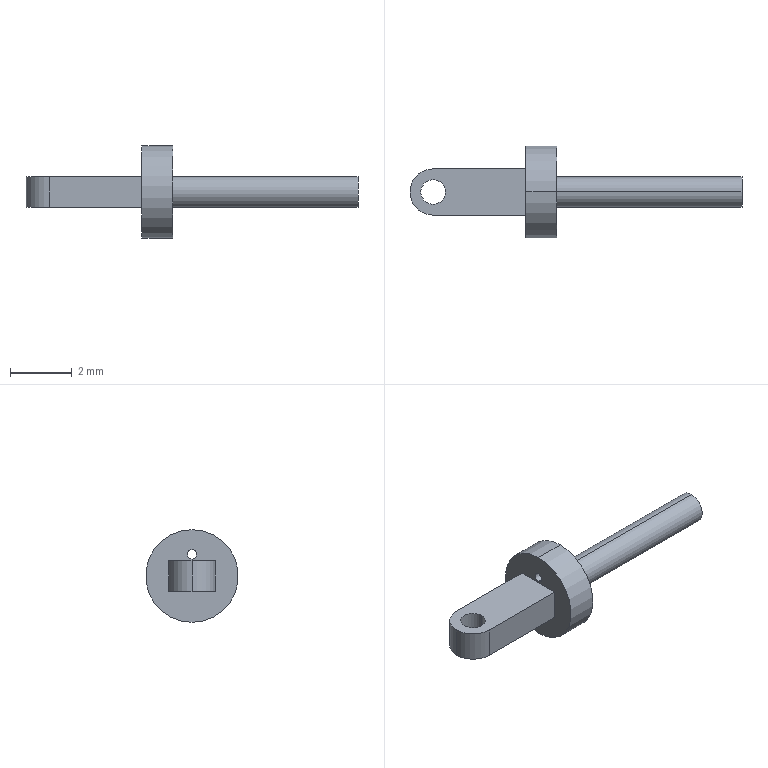Part | SolidWorks | features ICE 3, Revolution 1 | 1 solid | 17 faces | box 10.75 x 3 x 3 mm | volume 16.591 mm3 | cylinder 10 | plane 7 | commonest cylinder face diameters 0.3 x2 0.8 x2 1 x2 1.5 x2 3 x2
STEP:
#1=CARTESIAN_POINT('',(1.,0.,0.55));
#2=VERTEX_POINT('',#1);
#3=CARTESIAN_POINT('',(1.,0.,0.85));
#4=VERTEX_POINT('',#3);
#5=CARTESIAN_POINT('',(1.,0.,0.7));
#6=DIRECTION('',(-1.,0.,0.));
#7=DIRECTION('',(0.,0.,1.));
#8=AXIS2_PLACEMENT_3D('',#5,#6,#7);
#9=CIRCLE('',#8,0.15);
#10=EDGE_CURVE('',#2,#4,#9,.T.);
#11=ORIENTED_EDGE('',*,*,#10,.F.);
#12=CARTESIAN_POINT('',(0.,0.,0.55));
#13=VERTEX_POINT('',#12);
#14=CARTESIAN_POINT('',(10.,0.,0.55));
#15=DIRECTION('',(-1.,0.,0.));
#16=VECTOR('',#15,1000.);
#17=LINE('',#14,#16);
#18=EDGE_CURVE('',#2,#13,#17,.T.);
#19=ORIENTED_EDGE('',*,*,#18,.T.);
#20=CARTESIAN_POINT('',(0.,0.,0.85));
#21=VERTEX_POINT('',#20);
#22=CARTESIAN_POINT('',(0.,0.,0.7));
#23=DIRECTION('',(-1.,0.,0.));
#24=DIRECTION('',(0.,0.,1.));
#25=AXIS2_PLACEMENT_3D('',#22,#23,#24);
#26=CIRCLE('',#25,0.15);
#27=EDGE_CURVE('',#13,#21,#26,.T.);
#28=ORIENTED_EDGE('',*,*,#27,.T.);
#29=CARTESIAN_POINT('',(10.,0.,0.85));
#30=DIRECTION('',(-1.,0.,0.));
#31=VECTOR('',#30,1000.);
#32=LINE('',#29,#31);
#33=EDGE_CURVE('',#4,#21,#32,.T.);
#34=ORIENTED_EDGE('',*,*,#33,.F.);
#35=EDGE_LOOP('',(#11,#19,#28,#34));
#36=FACE_OUTER_BOUND('',#35,.T.);
#37=CARTESIAN_POINT('',(10.,0.,0.7));
#38=DIRECTION('',(-1.,0.,0.));
#39=DIRECTION('',(0.,0.,1.));
#40=AXIS2_PLACEMENT_3D('',#37,#38,#39);
#41=CYLINDRICAL_SURFACE('',#40,0.15);
#42=ADVANCED_FACE('',(#36),#41,.F.);
#43=CARTESIAN_POINT('',(1.,0.,-0.5));
#44=VERTEX_POINT('',#43);
#45=CARTESIAN_POINT('',(1.,0.,0.5));
#46=VERTEX_POINT('',#45);
#47=CARTESIAN_POINT('',(1.,0.,0.));
#48=DIRECTION('',(1.,0.,0.));
#49=DIRECTION('',(0.,0.,-1.));
#50=AXIS2_PLACEMENT_3D('',#47,#48,#49);
#51=CIRCLE('',#50,0.5);
#52=EDGE_CURVE('',#44,#46,#51,.T.);
#53=ORIENTED_EDGE('',*,*,#52,.T.);
#54=CARTESIAN_POINT('',(7.,0.,0.5));
#55=VERTEX_POINT('',#54);
#56=CARTESIAN_POINT('',(1.,0.,0.5));
#57=DIRECTION('',(1.,0.,0.));
#58=VECTOR('',#57,1000.);
#59=LINE('',#56,#58);
#60=EDGE_CURVE('',#46,#55,#59,.T.);
#61=ORIENTED_EDGE('',*,*,#60,.T.);
#62=CARTESIAN_POINT('',(7.,0.,-0.5));
#63=VERTEX_POINT('',#62);
#64=CARTESIAN_POINT('',(7.,0.,0.));
#65=DIRECTION('',(1.,0.,0.));
#66=DIRECTION('',(0.,0.,-1.));
#67=AXIS2_PLACEMENT_3D('',#64,#65,#66);
#68=CIRCLE('',#67,0.5);
#69=EDGE_CURVE('',#63,#55,#68,.T.);
#70=ORIENTED_EDGE('',*,*,#69,.F.);
#71=CARTESIAN_POINT('',(1.,0.,-0.5));
#72=DIRECTION('',(1.,0.,0.));
#73=VECTOR('',#72,1000.);
#74=LINE('',#71,#73);
#75=EDGE_CURVE('',#44,#63,#74,.T.);
#76=ORIENTED_EDGE('',*,*,#75,.F.);
#77=EDGE_LOOP('',(#53,#61,#70,#76));
#78=FACE_OUTER_BOUND('',#77,.T.);
#79=CARTESIAN_POINT('',(1.,0.,0.));
#80=DIRECTION('',(1.,0.,0.));
#81=DIRECTION('',(0.,0.,-1.));
#82=AXIS2_PLACEMENT_3D('',#79,#80,#81);
#83=CYLINDRICAL_SURFACE('',#82,0.5);
#84=ADVANCED_FACE('',(#78),#83,.T.);
#85=CARTESIAN_POINT('',(-3.4,0.,0.5));
#86=VERTEX_POINT('',#85);
#87=CARTESIAN_POINT('',(-2.6,0.,0.5));
#88=VERTEX_POINT('',#87);
#89=CARTESIAN_POINT('',(-3.,0.,0.5));
#90=DIRECTION('',(0.,0.,1.));
#91=DIRECTION('',(1.,0.,0.));
#92=AXIS2_PLACEMENT_3D('',#89,#90,#91);
#93=CIRCLE('',#92,0.4);
#94=EDGE_CURVE('',#86,#88,#93,.T.);
#95=ORIENTED_EDGE('',*,*,#94,.T.);
#96=CARTESIAN_POINT('',(-2.6,0.,-0.5));
#97=VERTEX_POINT('',#96);
#98=CARTESIAN_POINT('',(-2.6,0.,0.5));
#99=DIRECTION('',(0.,0.,-1.));
#100=VECTOR('',#99,1000.);
#101=LINE('',#98,#100);
#102=EDGE_CURVE('',#88,#97,#101,.T.);
#103=ORIENTED_EDGE('',*,*,#102,.T.);
#104=CARTESIAN_POINT('',(-3.4,0.,-0.5));
#105=VERTEX_POINT('',#104);
#106=CARTESIAN_POINT('',(-3.,0.,-0.5));
#107=DIRECTION('',(0.,0.,1.));
#108=DIRECTION('',(1.,0.,0.));
#109=AXIS2_PLACEMENT_3D('',#106,#107,#108);
#110=CIRCLE('',#109,0.4);
#111=EDGE_CURVE('',#105,#97,#110,.T.);
#112=ORIENTED_EDGE('',*,*,#111,.F.);
#113=CARTESIAN_POINT('',(-3.4,0.,0.5));
#114=DIRECTION('',(0.,0.,-1.));
#115=VECTOR('',#114,1000.);
#116=LINE('',#113,#115);
#117=EDGE_CURVE('',#86,#105,#116,.T.);
#118=ORIENTED_EDGE('',*,*,#117,.F.);
#119=EDGE_LOOP('',(#95,#103,#112,#118));
#120=FACE_OUTER_BOUND('',#119,.T.);
#121=CARTESIAN_POINT('',(-3.,0.,0.5));
#122=DIRECTION('',(0.,0.,-1.));
#123=DIRECTION('',(-1.,0.,0.));
#124=AXIS2_PLACEMENT_3D('',#121,#122,#123);
#125=CYLINDRICAL_SURFACE('',#124,0.4);
#126=ADVANCED_FACE('',(#120),#125,.F.);
#127=CARTESIAN_POINT('',(-3.75,0.,0.5));
#128=VERTEX_POINT('',#127);
#129=CARTESIAN_POINT('',(-3.,-0.75,0.5));
#130=VERTEX_POINT('',#129);
#131=CARTESIAN_POINT('',(-3.,0.,0.5));
#132=DIRECTION('',(0.,0.,1.));
#133=DIRECTION('',(-1.,0.,0.));
#134=AXIS2_PLACEMENT_3D('',#131,#132,#133);
#135=CIRCLE('',#134,0.75);
#136=EDGE_CURVE('',#128,#130,#135,.T.);
#137=ORIENTED_EDGE('',*,*,#136,.F.);
#138=CARTESIAN_POINT('',(-3.75,0.,-0.5));
#139=VERTEX_POINT('',#138);
#140=CARTESIAN_POINT('',(-3.75,0.,0.5));
#141=DIRECTION('',(0.,0.,-1.));
#142=VECTOR('',#141,1000.);
#143=LINE('',#140,#142);
#144=EDGE_CURVE('',#128,#139,#143,.T.);
#145=ORIENTED_EDGE('',*,*,#144,.T.);
#146=CARTESIAN_POINT('',(-3.,-0.75,-0.5));
#147=VERTEX_POINT('',#146);
#148=CARTESIAN_POINT('',(-3.,0.,-0.5));
#149=DIRECTION('',(0.,0.,1.));
#150=DIRECTION('',(-1.,0.,0.));
#151=AXIS2_PLACEMENT_3D('',#148,#149,#150);
#152=CIRCLE('',#151,0.75);
#153=EDGE_CURVE('',#139,#147,#152,.T.);
#154=ORIENTED_EDGE('',*,*,#153,.T.);
#155=CARTESIAN_POINT('',(-3.,-0.75,0.5));
#156=DIRECTION('',(0.,0.,-1.));
#157=VECTOR('',#156,1000.);
#158=LINE('',#155,#157);
#159=EDGE_CURVE('',#130,#147,#158,.T.);
#160=ORIENTED_EDGE('',*,*,#159,.F.);
#161=EDGE_LOOP('',(#137,#145,#154,#160));
#162=FACE_OUTER_BOUND('',#161,.T.);
#163=CARTESIAN_POINT('',(-3.,0.,0.5));
#164=DIRECTION('',(0.,0.,-1.));
#165=DIRECTION('',(-1.,0.,0.));
#166=AXIS2_PLACEMENT_3D('',#163,#164,#165);
#167=CYLINDRICAL_SURFACE('',#166,0.75);
#168=ADVANCED_FACE('',(#162),#167,.T.);
#169=CARTESIAN_POINT('',(1.,0.,1.5));
#170=VERTEX_POINT('',#169);
#171=CARTESIAN_POINT('',(1.,0.,-1.5));
#172=VERTEX_POINT('',#171);
#173=CARTESIAN_POINT('',(1.,0.,0.));
#174=DIRECTION('',(-1.,0.,0.));
#175=DIRECTION('',(0.,0.,1.));
#176=AXIS2_PLACEMENT_3D('',#173,#174,#175);
#177=CIRCLE('',#176,1.5);
#178=EDGE_CURVE('',#170,#172,#177,.T.);
#179=ORIENTED_EDGE('',*,*,#178,.T.);
#180=CARTESIAN_POINT('',(0.,0.,-1.5));
#181=VERTEX_POINT('',#180);
#182=CARTESIAN_POINT('',(0.1244,0.,-1.5));
#183=DIRECTION('',(-1.,0.,0.));
#184=VECTOR('',#183,1000.);
#185=LINE('',#182,#184);
#186=EDGE_CURVE('',#172,#181,#185,.T.);
#187=ORIENTED_EDGE('',*,*,#186,.T.);
#188=CARTESIAN_POINT('',(0.,0.,1.5));
#189=VERTEX_POINT('',#188);
#190=CARTESIAN_POINT('',(0.,0.,0.));
#191=DIRECTION('',(-1.,0.,0.));
#192=DIRECTION('',(0.,0.,1.));
#193=AXIS2_PLACEMENT_3D('',#190,#191,#192);
#194=CIRCLE('',#193,1.5);
#195=EDGE_CURVE('',#189,#181,#194,.T.);
#196=ORIENTED_EDGE('',*,*,#195,.F.);
#197=CARTESIAN_POINT('',(0.1244,0.,1.5));
#198=DIRECTION('',(-1.,0.,0.));
#199=VECTOR('',#198,1000.);
#200=LINE('',#197,#199);
#201=EDGE_CURVE('',#170,#189,#200,.T.);
#202=ORIENTED_EDGE('',*,*,#201,.F.);
#203=EDGE_LOOP('',(#179,#187,#196,#202));
#204=FACE_OUTER_BOUND('',#203,.T.);
#205=CARTESIAN_POINT('',(0.1244,0.,0.));
#206=DIRECTION('',(-1.,0.,0.));
#207=DIRECTION('',(0.,0.,1.));
#208=AXIS2_PLACEMENT_3D('',#205,#206,#207);
#209=CYLINDRICAL_SURFACE('',#208,1.5);
#210=ADVANCED_FACE('',(#204),#209,.T.);
#211=CARTESIAN_POINT('',(0.,0.,0.7));
#212=DIRECTION('',(-1.,0.,0.));
#213=DIRECTION('',(0.,0.,1.));
#214=AXIS2_PLACEMENT_3D('',#211,#212,#213);
#215=CIRCLE('',#214,0.15);
#216=EDGE_CURVE('',#21,#13,#215,.T.);
#217=ORIENTED_EDGE('',*,*,#216,.F.);
#218=ORIENTED_EDGE('',*,*,#27,.F.);
#219=EDGE_LOOP('',(#217,#218));
#220=FACE_BOUND('',#219,.T.);
#221=CARTESIAN_POINT('',(0.,-0.75,0.5));
#222=VERTEX_POINT('',#221);
#223=CARTESIAN_POINT('',(0.,-0.75,-0.5));
#224=VERTEX_POINT('',#223);
#225=CARTESIAN_POINT('',(0.,-0.75,0.5));
#226=DIRECTION('',(0.,0.,-1.));
#227=VECTOR('',#226,1000.);
#228=LINE('',#225,#227);
#229=EDGE_CURVE('',#222,#224,#228,.T.);
#230=ORIENTED_EDGE('',*,*,#229,.T.);
#231=CARTESIAN_POINT('',(0.,0.75,-0.5));
#232=VERTEX_POINT('',#231);
#233=CARTESIAN_POINT('',(0.,0.75,-0.5));
#234=DIRECTION('',(0.,1.,0.));
#235=VECTOR('',#234,1000.);
#236=LINE('',#233,#235);
#237=EDGE_CURVE('',#224,#232,#236,.T.);
#238=ORIENTED_EDGE('',*,*,#237,.T.);
#239=CARTESIAN_POINT('',(0.,0.75,0.5));
#240=VERTEX_POINT('',#239);
#241=CARTESIAN_POINT('',(0.,0.75,0.5));
#242=DIRECTION('',(0.,0.,-1.));
#243=VECTOR('',#242,1000.);
#244=LINE('',#241,#243);
#245=EDGE_CURVE('',#240,#232,#244,.T.);
#246=ORIENTED_EDGE('',*,*,#245,.F.);
#247=CARTESIAN_POINT('',(0.,0.75,0.5));
#248=DIRECTION('',(0.,1.,0.));
#249=VECTOR('',#248,1000.);
#250=LINE('',#247,#249);
#251=EDGE_CURVE('',#222,#240,#250,.T.);
#252=ORIENTED_EDGE('',*,*,#251,.F.);
#253=EDGE_LOOP('',(#230,#238,#246,#252));
#254=FACE_BOUND('',#253,.T.);
#255=ORIENTED_EDGE('',*,*,#195,.T.);
#256=CARTESIAN_POINT('',(0.,0.,0.));
#257=DIRECTION('',(-1.,0.,0.));
#258=DIRECTION('',(0.,0.,1.));
#259=AXIS2_PLACEMENT_3D('',#256,#257,#258);
#260=CIRCLE('',#259,1.5);
#261=EDGE_CURVE('',#181,#189,#260,.T.);
#262=ORIENTED_EDGE('',*,*,#261,.T.);
#263=EDGE_LOOP('',(#255,#262));
#264=FACE_OUTER_BOUND('',#263,.T.);
#265=CARTESIAN_POINT('',(0.,0.,0.));
#266=DIRECTION('',(1.,0.,0.));
#267=DIRECTION('',(0.,0.,-1.));
#268=AXIS2_PLACEMENT_3D('',#265,#266,#267);
#269=PLANE('',#268);
#270=ADVANCED_FACE('',(#220,#254,#264),#269,.F.);
#271=ORIENTED_EDGE('',*,*,#186,.F.);
#272=CARTESIAN_POINT('',(1.,0.,0.));
#273=DIRECTION('',(-1.,0.,0.));
#274=DIRECTION('',(0.,0.,1.));
#275=AXIS2_PLACEMENT_3D('',#272,#273,#274);
#276=CIRCLE('',#275,1.5);
#277=EDGE_CURVE('',#172,#170,#276,.T.);
#278=ORIENTED_EDGE('',*,*,#277,.T.);
#279=ORIENTED_EDGE('',*,*,#201,.T.);
#280=ORIENTED_EDGE('',*,*,#261,.F.);
#281=EDGE_LOOP('',(#271,#278,#279,#280));
#282=FACE_OUTER_BOUND('',#281,.T.);
#283=CARTESIAN_POINT('',(0.1244,0.,0.));
#284=DIRECTION('',(-1.,0.,0.));
#285=DIRECTION('',(0.,0.,1.));
#286=AXIS2_PLACEMENT_3D('',#283,#284,#285);
#287=CYLINDRICAL_SURFACE('',#286,1.5);
#288=ADVANCED_FACE('',(#282),#287,.T.);
#289=CARTESIAN_POINT('',(1.,0.,0.7));
#290=DIRECTION('',(-1.,0.,0.));
#291=DIRECTION('',(0.,0.,1.));
#292=AXIS2_PLACEMENT_3D('',#289,#290,#291);
#293=CIRCLE('',#292,0.15);
#294=EDGE_CURVE('',#4,#2,#293,.T.);
#295=ORIENTED_EDGE('',*,*,#294,.T.);
#296=ORIENTED_EDGE('',*,*,#10,.T.);
#297=EDGE_LOOP('',(#295,#296));
#298=FACE_BOUND('',#297,.T.);
#299=ORIENTED_EDGE('',*,*,#178,.F.);
#300=ORIENTED_EDGE('',*,*,#277,.F.);
#301=EDGE_LOOP('',(#299,#300));
#302=FACE_OUTER_BOUND('',#301,.T.);
#303=ORIENTED_EDGE('',*,*,#52,.F.);
#304=CARTESIAN_POINT('',(1.,0.,0.));
#305=DIRECTION('',(1.,0.,0.));
#306=DIRECTION('',(0.,0.,-1.));
#307=AXIS2_PLACEMENT_3D('',#304,#305,#306);
#308=CIRCLE('',#307,0.5);
#309=EDGE_CURVE('',#46,#44,#308,.T.);
#310=ORIENTED_EDGE('',*,*,#309,.F.);
#311=EDGE_LOOP('',(#303,#310));
#312=FACE_BOUND('',#311,.T.);
#313=CARTESIAN_POINT('',(1.,1.5,0.));
#314=DIRECTION('',(-1.,0.,0.));
#315=DIRECTION('',(0.,0.,1.));
#316=AXIS2_PLACEMENT_3D('',#313,#314,#315);
#317=PLANE('',#316);
#318=ADVANCED_FACE('',(#298,#302,#312),#317,.F.);
#319=CARTESIAN_POINT('',(0.,-0.75,0.5));
#320=DIRECTION('',(1.,0.,0.));
#321=VECTOR('',#320,1000.);
#322=LINE('',#319,#321);
#323=EDGE_CURVE('',#130,#222,#322,.T.);
#324=ORIENTED_EDGE('',*,*,#323,.T.);
#325=ORIENTED_EDGE('',*,*,#251,.T.);
#326=CARTESIAN_POINT('',(-3.,0.75,0.5));
#327=VERTEX_POINT('',#326);
#328=CARTESIAN_POINT('',(0.,0.75,0.5));
#329=DIRECTION('',(-1.,0.,0.));
#330=VECTOR('',#329,1000.);
#331=LINE('',#328,#330);
#332=EDGE_CURVE('',#240,#327,#331,.T.);
#333=ORIENTED_EDGE('',*,*,#332,.T.);
#334=CARTESIAN_POINT('',(-3.,0.,0.5));
#335=DIRECTION('',(0.,0.,1.));
#336=DIRECTION('',(-1.,0.,0.));
#337=AXIS2_PLACEMENT_3D('',#334,#335,#336);
#338=CIRCLE('',#337,0.75);
#339=EDGE_CURVE('',#327,#128,#338,.T.);
#340=ORIENTED_EDGE('',*,*,#339,.T.);
#341=ORIENTED_EDGE('',*,*,#136,.T.);
#342=EDGE_LOOP('',(#324,#325,#333,#340,#341));
#343=FACE_OUTER_BOUND('',#342,.T.);
#344=ORIENTED_EDGE('',*,*,#94,.F.);
#345=CARTESIAN_POINT('',(-3.,0.,0.5));
#346=DIRECTION('',(0.,0.,1.));
#347=DIRECTION('',(1.,0.,0.));
#348=AXIS2_PLACEMENT_3D('',#345,#346,#347);
#349=CIRCLE('',#348,0.4);
#350=EDGE_CURVE('',#88,#86,#349,.T.);
#351=ORIENTED_EDGE('',*,*,#350,.F.);
#352=EDGE_LOOP('',(#344,#351));
#353=FACE_BOUND('',#352,.T.);
#354=CARTESIAN_POINT('',(-3.,0.,0.5));
#355=DIRECTION('',(0.,0.,-1.));
#356=DIRECTION('',(-1.,0.,0.));
#357=AXIS2_PLACEMENT_3D('',#354,#355,#356);
#358=PLANE('',#357);
#359=ADVANCED_FACE('',(#343,#353),#358,.F.);
#360=CARTESIAN_POINT('',(0.,-0.75,-0.5));
#361=DIRECTION('',(1.,0.,0.));
#362=VECTOR('',#361,1000.);
#363=LINE('',#360,#362);
#364=EDGE_CURVE('',#147,#224,#363,.T.);
#365=ORIENTED_EDGE('',*,*,#364,.F.);
#366=ORIENTED_EDGE('',*,*,#153,.F.);
#367=CARTESIAN_POINT('',(-3.,0.75,-0.5));
#368=VERTEX_POINT('',#367);
#369=CARTESIAN_POINT('',(-3.,0.,-0.5));
#370=DIRECTION('',(0.,0.,1.));
#371=DIRECTION('',(-1.,0.,0.));
#372=AXIS2_PLACEMENT_3D('',#369,#370,#371);
#373=CIRCLE('',#372,0.75);
#374=EDGE_CURVE('',#368,#139,#373,.T.);
#375=ORIENTED_EDGE('',*,*,#374,.F.);
#376=CARTESIAN_POINT('',(0.,0.75,-0.5));
#377=DIRECTION('',(-1.,0.,0.));
#378=VECTOR('',#377,1000.);
#379=LINE('',#376,#378);
#380=EDGE_CURVE('',#232,#368,#379,.T.);
#381=ORIENTED_EDGE('',*,*,#380,.F.);
#382=ORIENTED_EDGE('',*,*,#237,.F.);
#383=EDGE_LOOP('',(#365,#366,#375,#381,#382));
#384=FACE_OUTER_BOUND('',#383,.T.);
#385=ORIENTED_EDGE('',*,*,#111,.T.);
#386=CARTESIAN_POINT('',(-3.,0.,-0.5));
#387=DIRECTION('',(0.,0.,1.));
#388=DIRECTION('',(1.,0.,0.));
#389=AXIS2_PLACEMENT_3D('',#386,#387,#388);
#390=CIRCLE('',#389,0.4);
#391=EDGE_CURVE('',#97,#105,#390,.T.);
#392=ORIENTED_EDGE('',*,*,#391,.T.);
#393=EDGE_LOOP('',(#385,#392));
#394=FACE_BOUND('',#393,.T.);
#395=CARTESIAN_POINT('',(-3.,0.,-0.5));
#396=DIRECTION('',(0.,0.,-1.));
#397=DIRECTION('',(-1.,0.,0.));
#398=AXIS2_PLACEMENT_3D('',#395,#396,#397);
#399=PLANE('',#398);
#400=ADVANCED_FACE('',(#384,#394),#399,.T.);
#401=ORIENTED_EDGE('',*,*,#364,.T.);
#402=ORIENTED_EDGE('',*,*,#229,.F.);
#403=ORIENTED_EDGE('',*,*,#323,.F.);
#404=ORIENTED_EDGE('',*,*,#159,.T.);
#405=EDGE_LOOP('',(#401,#402,#403,#404));
#406=FACE_OUTER_BOUND('',#405,.T.);
#407=CARTESIAN_POINT('',(0.,-0.75,0.5));
#408=DIRECTION('',(0.,1.,0.));
#409=DIRECTION('',(-1.,0.,0.));
#410=AXIS2_PLACEMENT_3D('',#407,#408,#409);
#411=PLANE('',#410);
#412=ADVANCED_FACE('',(#406),#411,.F.);
#413=ORIENTED_EDGE('',*,*,#380,.T.);
#414=CARTESIAN_POINT('',(-3.,0.75,0.5));
#415=DIRECTION('',(0.,0.,-1.));
#416=VECTOR('',#415,1000.);
#417=LINE('',#414,#416);
#418=EDGE_CURVE('',#327,#368,#417,.T.);
#419=ORIENTED_EDGE('',*,*,#418,.F.);
#420=ORIENTED_EDGE('',*,*,#332,.F.);
#421=ORIENTED_EDGE('',*,*,#245,.T.);
#422=EDGE_LOOP('',(#413,#419,#420,#421));
#423=FACE_OUTER_BOUND('',#422,.T.);
#424=CARTESIAN_POINT('',(0.,0.75,0.5));
#425=DIRECTION('',(0.,-1.,0.));
#426=DIRECTION('',(1.,0.,0.));
#427=AXIS2_PLACEMENT_3D('',#424,#425,#426);
#428=PLANE('',#427);
#429=ADVANCED_FACE('',(#423),#428,.F.);
#430=ORIENTED_EDGE('',*,*,#144,.F.);
#431=ORIENTED_EDGE('',*,*,#339,.F.);
#432=ORIENTED_EDGE('',*,*,#418,.T.);
#433=ORIENTED_EDGE('',*,*,#374,.T.);
#434=EDGE_LOOP('',(#430,#431,#432,#433));
#435=FACE_OUTER_BOUND('',#434,.T.);
#436=CARTESIAN_POINT('',(-3.,0.,0.5));
#437=DIRECTION('',(0.,0.,-1.));
#438=DIRECTION('',(-1.,0.,0.));
#439=AXIS2_PLACEMENT_3D('',#436,#437,#438);
#440=CYLINDRICAL_SURFACE('',#439,0.75);
#441=ADVANCED_FACE('',(#435),#440,.T.);
#442=ORIENTED_EDGE('',*,*,#102,.F.);
#443=ORIENTED_EDGE('',*,*,#350,.T.);
#444=ORIENTED_EDGE('',*,*,#117,.T.);
#445=ORIENTED_EDGE('',*,*,#391,.F.);
#446=EDGE_LOOP('',(#442,#443,#444,#445));
#447=FACE_OUTER_BOUND('',#446,.T.);
#448=CARTESIAN_POINT('',(-3.,0.,0.5));
#449=DIRECTION('',(0.,0.,-1.));
#450=DIRECTION('',(-1.,0.,0.));
#451=AXIS2_PLACEMENT_3D('',#448,#449,#450);
#452=CYLINDRICAL_SURFACE('',#451,0.4);
#453=ADVANCED_FACE('',(#447),#452,.F.);
#454=ORIENTED_EDGE('',*,*,#60,.F.);
#455=ORIENTED_EDGE('',*,*,#309,.T.);
#456=ORIENTED_EDGE('',*,*,#75,.T.);
#457=CARTESIAN_POINT('',(7.,0.,0.));
#458=DIRECTION('',(1.,0.,0.));
#459=DIRECTION('',(0.,0.,-1.));
#460=AXIS2_PLACEMENT_3D('',#457,#458,#459);
#461=CIRCLE('',#460,0.5);
#462=EDGE_CURVE('',#55,#63,#461,.T.);
#463=ORIENTED_EDGE('',*,*,#462,.F.);
#464=EDGE_LOOP('',(#454,#455,#456,#463));
#465=FACE_OUTER_BOUND('',#464,.T.);
#466=CARTESIAN_POINT('',(1.,0.,0.));
#467=DIRECTION('',(1.,0.,0.));
#468=DIRECTION('',(0.,0.,-1.));
#469=AXIS2_PLACEMENT_3D('',#466,#467,#468);
#470=CYLINDRICAL_SURFACE('',#469,0.5);
#471=ADVANCED_FACE('',(#465),#470,.T.);
#472=ORIENTED_EDGE('',*,*,#69,.T.);
#473=ORIENTED_EDGE('',*,*,#462,.T.);
#474=EDGE_LOOP('',(#472,#473));
#475=FACE_OUTER_BOUND('',#474,.T.);
#476=CARTESIAN_POINT('',(7.,1.,0.));
#477=DIRECTION('',(-1.,0.,0.));
#478=DIRECTION('',(0.,0.,1.));
#479=AXIS2_PLACEMENT_3D('',#476,#477,#478);
#480=PLANE('',#479);
#481=ADVANCED_FACE('',(#475),#480,.F.);
#482=ORIENTED_EDGE('',*,*,#18,.F.);
#483=ORIENTED_EDGE('',*,*,#294,.F.);
#484=ORIENTED_EDGE('',*,*,#33,.T.);
#485=ORIENTED_EDGE('',*,*,#216,.T.);
#486=EDGE_LOOP('',(#482,#483,#484,#485));
#487=FACE_OUTER_BOUND('',#486,.T.);
#488=CARTESIAN_POINT('',(10.,0.,0.7));
#489=DIRECTION('',(-1.,0.,0.));
#490=DIRECTION('',(0.,0.,1.));
#491=AXIS2_PLACEMENT_3D('',#488,#489,#490);
#492=CYLINDRICAL_SURFACE('',#491,0.15);
#493=ADVANCED_FACE('',(#487),#492,.F.);
#494=CLOSED_SHELL('',(#42,#84,#126,#168,#210,#270,#288,#318,#359,#400,#412,#429,#441,#453,#471,#481,#493));
#495=MANIFOLD_SOLID_BREP('',#494);
#496=CARTESIAN_POINT('',(0.,0.,0.));
#497=DIRECTION('',(0.,0.,1.));
#498=DIRECTION('',(1.,0.,0.));
#499=AXIS2_PLACEMENT_3D('',#496,#497,#498);
#500=(LENGTH_UNIT()NAMED_UNIT(*)SI_UNIT(.MILLI.,.METRE.));
#501=UNCERTAINTY_MEASURE_WITH_UNIT(LENGTH_MEASURE(0.00001),#500,'','');
#502=(NAMED_UNIT(*)PLANE_ANGLE_UNIT()SI_UNIT($,.RADIAN.));
#503=(NAMED_UNIT(*)SI_UNIT($,.STERADIAN.)SOLID_ANGLE_UNIT());
#504=(GEOMETRIC_REPRESENTATION_CONTEXT(3)GLOBAL_UNCERTAINTY_ASSIGNED_CONTEXT((#501))GLOBAL_UNIT_ASSIGNED_CONTEXT((#500,#502,#503))REPRESENTATION_CONTEXT('',''));
#505=ADVANCED_BREP_SHAPE_REPRESENTATION('',(#495,#499),#504);